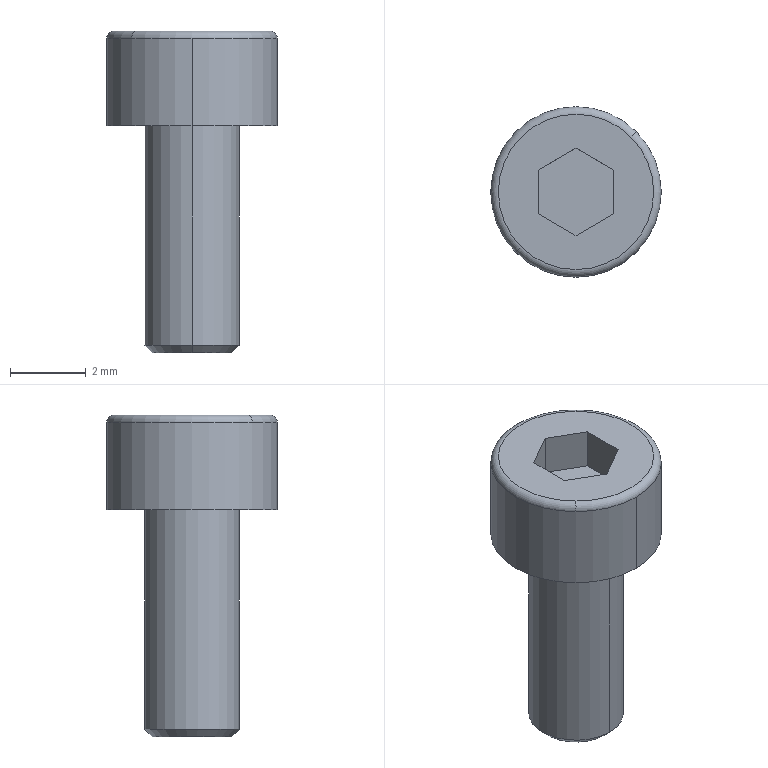Part | STEP file | ASND-0110-0211110266 | 1 solid | 18 faces | box 4.5 x 4.5 x 8.5 mm | volume 65.135 mm3 | plane 10 | cylinder 4 | torus 2 | cone 2 | commonest cylinder face diameters 2.5 x2 4.5 x2
STEP:
#1=CARTESIAN_POINT('',(0.,0.,0.));
#2=DIRECTION('',(0.,0.,1.));
#3=DIRECTION('',(1.,0.,0.));
#4=AXIS2_PLACEMENT_3D('',#1,#2,#3);
#5=CARTESIAN_POINT('',(-1.45,-1.45,2.5));
#6=VERTEX_POINT('',#5);
#7=CARTESIAN_POINT('',(1.45,1.45,2.5));
#8=VERTEX_POINT('',#7);
#9=CARTESIAN_POINT('',(0.,0.,2.5));
#10=DIRECTION('',(0.,0.,1.));
#11=DIRECTION('',(0.,-1.,0.));
#12=AXIS2_PLACEMENT_3D('',#9,#10,#11);
#13=CIRCLE('',#12,2.05);
#14=CARTESIAN_POINT('',(0.,0.,2.3));
#15=DIRECTION('',(0.,0.,-1.));
#16=DIRECTION('',(0.7071,0.7071,0.));
#17=AXIS2_PLACEMENT_3D('',#14,#15,#16);
#18=TOROIDAL_SURFACE('',#17,2.05,0.2);
#19=CARTESIAN_POINT('',(8.639,4.712));
#20=DIRECTION('',(-1.,0.));
#21=VECTOR('',#20,1.);
#22=LINE('',#19,#21);
#23=(GEOMETRIC_REPRESENTATION_CONTEXT(2)PARAMETRIC_REPRESENTATION_CONTEXT()REPRESENTATION_CONTEXT('',''));
#24=DEFINITIONAL_REPRESENTATION('',(#22),#23);
#25=PCURVE('',#18,#24);
#26=CARTESIAN_POINT('',(0.,0.,2.5));
#27=DIRECTION('',(0.,0.,-1.));
#28=DIRECTION('',(0.7071,0.7071,0.));
#29=AXIS2_PLACEMENT_3D('',#26,#27,#28);
#30=PLANE('',#29);
#31=CARTESIAN_POINT('',(-1.45,1.45));
#32=CARTESIAN_POINT('',(1.061,3.96));
#33=CARTESIAN_POINT('',(1.98,0.5306));
#34=CARTESIAN_POINT('',(2.899,-2.899));
#35=CARTESIAN_POINT('',(-0.5306,-1.98));
#36=CARTESIAN_POINT('',(-3.96,-1.061));
#37=CARTESIAN_POINT('',(-1.45,1.45));
#38=(BOUNDED_CURVE()B_SPLINE_CURVE(2,(#31,#32,#33,#34,#35,#36,#37),.UNSPECIFIED.,.T.,.F.)B_SPLINE_CURVE_WITH_KNOTS((1,2,2,2,2,1),(-2.094,0.,2.094,4.189,6.283,8.378),.UNSPECIFIED.)CURVE()GEOMETRIC_REPRESENTATION_ITEM()RATIONAL_B_SPLINE_CURVE((1.,0.5,1.,0.5,1.,0.5,1.))REPRESENTATION_ITEM(''));
#39=(GEOMETRIC_REPRESENTATION_CONTEXT(2)PARAMETRIC_REPRESENTATION_CONTEXT()REPRESENTATION_CONTEXT('',''));
#40=DEFINITIONAL_REPRESENTATION('',(#38),#39);
#41=PCURVE('',#30,#40);
#42=SURFACE_CURVE('',#13,(#25,#41),.PCURVE_S1.);
#43=EDGE_CURVE('',#6,#8,#42,.T.);
#44=ORIENTED_EDGE('',*,*,#43,.F.);
#45=CARTESIAN_POINT('',(-1.591,-1.591,2.3));
#46=VERTEX_POINT('',#45);
#47=CARTESIAN_POINT('',(-1.45,-1.45,2.3));
#48=DIRECTION('',(0.7071,-0.7071,0.));
#49=DIRECTION('',(0.7071,0.7071,0.));
#50=AXIS2_PLACEMENT_3D('',#47,#48,#49);
#51=CIRCLE('',#50,0.2);
#52=CARTESIAN_POINT('',(3.142,3.142));
#53=DIRECTION('',(0.,1.));
#54=VECTOR('',#53,1.);
#55=LINE('',#52,#54);
#56=(GEOMETRIC_REPRESENTATION_CONTEXT(2)PARAMETRIC_REPRESENTATION_CONTEXT()REPRESENTATION_CONTEXT('',''));
#57=DEFINITIONAL_REPRESENTATION('',(#55),#56);
#58=PCURVE('',#18,#57);
#59=CARTESIAN_POINT('',(0.,0.,2.3));
#60=DIRECTION('',(0.,0.,-1.));
#61=DIRECTION('',(0.7071,0.7071,0.));
#62=AXIS2_PLACEMENT_3D('',#59,#60,#61);
#63=TOROIDAL_SURFACE('',#62,2.05,0.2);
#64=CARTESIAN_POINT('',(3.142,3.142));
#65=DIRECTION('',(0.,1.));
#66=VECTOR('',#65,1.);
#67=LINE('',#64,#66);
#68=(GEOMETRIC_REPRESENTATION_CONTEXT(2)PARAMETRIC_REPRESENTATION_CONTEXT()REPRESENTATION_CONTEXT('',''));
#69=DEFINITIONAL_REPRESENTATION('',(#67),#68);
#70=PCURVE('',#63,#69);
#71=SURFACE_CURVE('',#51,(#58,#70),.PCURVE_S1.);
#72=EDGE_CURVE('',#6,#46,#71,.T.);
#73=ORIENTED_EDGE('',*,*,#72,.T.);
#74=CARTESIAN_POINT('',(0.,-2.25,2.3));
#75=VERTEX_POINT('',#74);
#76=CARTESIAN_POINT('',(0.,0.,2.3));
#77=DIRECTION('',(0.,0.,1.));
#78=DIRECTION('',(0.,-1.,0.));
#79=AXIS2_PLACEMENT_3D('',#76,#77,#78);
#80=CIRCLE('',#79,2.25);
#81=CARTESIAN_POINT('',(8.639,6.283));
#82=DIRECTION('',(-1.,0.));
#83=VECTOR('',#82,1.);
#84=LINE('',#81,#83);
#85=(GEOMETRIC_REPRESENTATION_CONTEXT(2)PARAMETRIC_REPRESENTATION_CONTEXT()REPRESENTATION_CONTEXT('',''));
#86=DEFINITIONAL_REPRESENTATION('',(#84),#85);
#87=PCURVE('',#18,#86);
#88=CARTESIAN_POINT('',(0.,0.,2.925));
#89=DIRECTION('',(0.,0.,-1.));
#90=DIRECTION('',(0.,1.,0.));
#91=AXIS2_PLACEMENT_3D('',#88,#89,#90);
#92=CYLINDRICAL_SURFACE('',#91,2.25);
#93=CARTESIAN_POINT('',(9.425,0.625));
#94=DIRECTION('',(-1.,0.));
#95=VECTOR('',#94,1.);
#96=LINE('',#93,#95);
#97=(GEOMETRIC_REPRESENTATION_CONTEXT(2)PARAMETRIC_REPRESENTATION_CONTEXT()REPRESENTATION_CONTEXT('',''));
#98=DEFINITIONAL_REPRESENTATION('',(#96),#97);
#99=PCURVE('',#92,#98);
#100=SURFACE_CURVE('',#80,(#87,#99),.PCURVE_S1.);
#101=EDGE_CURVE('',#46,#75,#100,.T.);
#102=ORIENTED_EDGE('',*,*,#101,.T.);
#103=CARTESIAN_POINT('',(1.591,1.591,2.3));
#104=VERTEX_POINT('',#103);
#105=CARTESIAN_POINT('',(0.,0.,2.3));
#106=DIRECTION('',(0.,0.,1.));
#107=DIRECTION('',(0.,-1.,0.));
#108=AXIS2_PLACEMENT_3D('',#105,#106,#107);
#109=CIRCLE('',#108,2.25);
#110=CARTESIAN_POINT('',(2.356,6.283));
#111=DIRECTION('',(-1.,0.));
#112=VECTOR('',#111,1.);
#113=LINE('',#110,#112);
#114=(GEOMETRIC_REPRESENTATION_CONTEXT(2)PARAMETRIC_REPRESENTATION_CONTEXT()REPRESENTATION_CONTEXT('',''));
#115=DEFINITIONAL_REPRESENTATION('',(#113),#114);
#116=PCURVE('',#18,#115);
#117=CARTESIAN_POINT('',(0.,0.,2.925));
#118=DIRECTION('',(0.,0.,-1.));
#119=DIRECTION('',(0.,1.,0.));
#120=AXIS2_PLACEMENT_3D('',#117,#118,#119);
#121=CYLINDRICAL_SURFACE('',#120,2.25);
#122=CARTESIAN_POINT('',(3.142,0.625));
#123=DIRECTION('',(-1.,0.));
#124=VECTOR('',#123,1.);
#125=LINE('',#122,#124);
#126=(GEOMETRIC_REPRESENTATION_CONTEXT(2)PARAMETRIC_REPRESENTATION_CONTEXT()REPRESENTATION_CONTEXT('',''));
#127=DEFINITIONAL_REPRESENTATION('',(#125),#126);
#128=PCURVE('',#121,#127);
#129=SURFACE_CURVE('',#109,(#116,#128),.PCURVE_S1.);
#130=EDGE_CURVE('',#75,#104,#129,.T.);
#131=ORIENTED_EDGE('',*,*,#130,.T.);
#132=CARTESIAN_POINT('',(1.45,1.45,2.3));
#133=DIRECTION('',(-0.7071,0.7071,0.));
#134=DIRECTION('',(-0.7071,-0.7071,0.));
#135=AXIS2_PLACEMENT_3D('',#132,#133,#134);
#136=CIRCLE('',#135,0.2);
#137=CARTESIAN_POINT('',(0.,3.142));
#138=DIRECTION('',(0.,1.));
#139=VECTOR('',#138,1.);
#140=LINE('',#137,#139);
#141=(GEOMETRIC_REPRESENTATION_CONTEXT(2)PARAMETRIC_REPRESENTATION_CONTEXT()REPRESENTATION_CONTEXT('',''));
#142=DEFINITIONAL_REPRESENTATION('',(#140),#141);
#143=PCURVE('',#18,#142);
#144=CARTESIAN_POINT('',(6.283,3.142));
#145=DIRECTION('',(0.,1.));
#146=VECTOR('',#145,1.);
#147=LINE('',#144,#146);
#148=(GEOMETRIC_REPRESENTATION_CONTEXT(2)PARAMETRIC_REPRESENTATION_CONTEXT()REPRESENTATION_CONTEXT('',''));
#149=DEFINITIONAL_REPRESENTATION('',(#147),#148);
#150=PCURVE('',#63,#149);
#151=SURFACE_CURVE('',#136,(#143,#150),.PCURVE_S1.);
#152=EDGE_CURVE('',#8,#104,#151,.T.);
#153=ORIENTED_EDGE('',*,*,#152,.F.);
#154=EDGE_LOOP('',(#44,#73,#102,#131,#153));
#155=FACE_BOUND('',#154,.T.);
#156=ADVANCED_FACE('',(#155),#18,.T.);
#157=ORIENTED_EDGE('',*,*,#130,.F.);
#158=CARTESIAN_POINT('',(0.,-2.25,0.));
#159=VERTEX_POINT('',#158);
#160=CARTESIAN_POINT('',(0.,-2.25,2.925));
#161=DIRECTION('',(0.,0.,-1.));
#162=VECTOR('',#161,1.);
#163=LINE('',#160,#162);
#164=CARTESIAN_POINT('',(3.142,0.));
#165=DIRECTION('',(0.,1.));
#166=VECTOR('',#165,1.);
#167=LINE('',#164,#166);
#168=(GEOMETRIC_REPRESENTATION_CONTEXT(2)PARAMETRIC_REPRESENTATION_CONTEXT()REPRESENTATION_CONTEXT('',''));
#169=DEFINITIONAL_REPRESENTATION('',(#167),#168);
#170=PCURVE('',#121,#169);
#171=CARTESIAN_POINT('',(3.142,0.));
#172=DIRECTION('',(0.,1.));
#173=VECTOR('',#172,1.);
#174=LINE('',#171,#173);
#175=(GEOMETRIC_REPRESENTATION_CONTEXT(2)PARAMETRIC_REPRESENTATION_CONTEXT()REPRESENTATION_CONTEXT('',''));
#176=DEFINITIONAL_REPRESENTATION('',(#174),#175);
#177=PCURVE('',#92,#176);
#178=SURFACE_CURVE('',#163,(#170,#177),.PCURVE_S1.);
#179=EDGE_CURVE('',#75,#159,#178,.T.);
#180=ORIENTED_EDGE('',*,*,#179,.T.);
#181=CARTESIAN_POINT('',(0.,2.25,0.));
#182=VERTEX_POINT('',#181);
#183=CARTESIAN_POINT('',(0.,0.,0.));
#184=DIRECTION('',(0.,0.,1.));
#185=DIRECTION('',(0.,-1.,0.));
#186=AXIS2_PLACEMENT_3D('',#183,#184,#185);
#187=CIRCLE('',#186,2.25);
#188=CARTESIAN_POINT('',(3.142,2.925));
#189=DIRECTION('',(-1.,0.));
#190=VECTOR('',#189,1.);
#191=LINE('',#188,#190);
#192=(GEOMETRIC_REPRESENTATION_CONTEXT(2)PARAMETRIC_REPRESENTATION_CONTEXT()REPRESENTATION_CONTEXT('',''));
#193=DEFINITIONAL_REPRESENTATION('',(#191),#192);
#194=PCURVE('',#121,#193);
#195=CARTESIAN_POINT('',(0.,0.,0.));
#196=DIRECTION('',(0.,0.,-1.));
#197=DIRECTION('',(0.7071,0.7071,0.));
#198=AXIS2_PLACEMENT_3D('',#195,#196,#197);
#199=PLANE('',#198);
#200=CARTESIAN_POINT('',(-1.591,1.591));
#201=CARTESIAN_POINT('',(1.165,4.347));
#202=CARTESIAN_POINT('',(2.173,0.5823));
#203=CARTESIAN_POINT('',(3.182,-3.182));
#204=CARTESIAN_POINT('',(-0.5823,-2.173));
#205=CARTESIAN_POINT('',(-4.347,-1.165));
#206=CARTESIAN_POINT('',(-1.591,1.591));
#207=(BOUNDED_CURVE()B_SPLINE_CURVE(2,(#200,#201,#202,#203,#204,#205,#206),.UNSPECIFIED.,.T.,.F.)B_SPLINE_CURVE_WITH_KNOTS((1,2,2,2,2,1),(-2.094,0.,2.094,4.189,6.283,8.378),.UNSPECIFIED.)CURVE()GEOMETRIC_REPRESENTATION_ITEM()RATIONAL_B_SPLINE_CURVE((1.,0.5,1.,0.5,1.,0.5,1.))REPRESENTATION_ITEM(''));
#208=(GEOMETRIC_REPRESENTATION_CONTEXT(2)PARAMETRIC_REPRESENTATION_CONTEXT()REPRESENTATION_CONTEXT('',''));
#209=DEFINITIONAL_REPRESENTATION('',(#207),#208);
#210=PCURVE('',#199,#209);
#211=SURFACE_CURVE('',#187,(#194,#210),.PCURVE_S1.);
#212=EDGE_CURVE('',#159,#182,#211,.T.);
#213=ORIENTED_EDGE('',*,*,#212,.T.);
#214=CARTESIAN_POINT('',(0.,2.25,2.3));
#215=VERTEX_POINT('',#214);
#216=CARTESIAN_POINT('',(0.,2.25,2.925));
#217=DIRECTION('',(0.,0.,-1.));
#218=VECTOR('',#217,1.);
#219=LINE('',#216,#218);
#220=CARTESIAN_POINT('',(0.,0.));
#221=DIRECTION('',(0.,1.));
#222=VECTOR('',#221,1.);
#223=LINE('',#220,#222);
#224=(GEOMETRIC_REPRESENTATION_CONTEXT(2)PARAMETRIC_REPRESENTATION_CONTEXT()REPRESENTATION_CONTEXT('',''));
#225=DEFINITIONAL_REPRESENTATION('',(#223),#224);
#226=PCURVE('',#121,#225);
#227=CARTESIAN_POINT('',(6.283,0.));
#228=DIRECTION('',(0.,1.));
#229=VECTOR('',#228,1.);
#230=LINE('',#227,#229);
#231=(GEOMETRIC_REPRESENTATION_CONTEXT(2)PARAMETRIC_REPRESENTATION_CONTEXT()REPRESENTATION_CONTEXT('',''));
#232=DEFINITIONAL_REPRESENTATION('',(#230),#231);
#233=PCURVE('',#92,#232);
#234=SURFACE_CURVE('',#219,(#226,#233),.PCURVE_S1.);
#235=EDGE_CURVE('',#215,#182,#234,.T.);
#236=ORIENTED_EDGE('',*,*,#235,.F.);
#237=CARTESIAN_POINT('',(0.,0.,2.3));
#238=DIRECTION('',(0.,0.,1.));
#239=DIRECTION('',(0.,-1.,0.));
#240=AXIS2_PLACEMENT_3D('',#237,#238,#239);
#241=CIRCLE('',#240,2.25);
#242=CARTESIAN_POINT('',(3.142,0.625));
#243=DIRECTION('',(-1.,0.));
#244=VECTOR('',#243,1.);
#245=LINE('',#242,#244);
#246=(GEOMETRIC_REPRESENTATION_CONTEXT(2)PARAMETRIC_REPRESENTATION_CONTEXT()REPRESENTATION_CONTEXT('',''));
#247=DEFINITIONAL_REPRESENTATION('',(#245),#246);
#248=PCURVE('',#121,#247);
#249=CARTESIAN_POINT('',(8.639,6.283));
#250=DIRECTION('',(-1.,0.));
#251=VECTOR('',#250,1.);
#252=LINE('',#249,#251);
#253=(GEOMETRIC_REPRESENTATION_CONTEXT(2)PARAMETRIC_REPRESENTATION_CONTEXT()REPRESENTATION_CONTEXT('',''));
#254=DEFINITIONAL_REPRESENTATION('',(#252),#253);
#255=PCURVE('',#63,#254);
#256=SURFACE_CURVE('',#241,(#248,#255),.PCURVE_S1.);
#257=EDGE_CURVE('',#104,#215,#256,.T.);
#258=ORIENTED_EDGE('',*,*,#257,.F.);
#259=EDGE_LOOP('',(#157,#180,#213,#236,#258));
#260=FACE_BOUND('',#259,.T.);
#261=ADVANCED_FACE('',(#260),#121,.T.);
#262=CARTESIAN_POINT('',(0.,1.25,0.));
#263=VERTEX_POINT('',#262);
#264=CARTESIAN_POINT('',(0.,-1.25,0.));
#265=VERTEX_POINT('',#264);
#266=CARTESIAN_POINT('',(0.,0.,0.));
#267=DIRECTION('',(0.,0.,-1.));
#268=DIRECTION('',(0.,-1.,0.));
#269=AXIS2_PLACEMENT_3D('',#266,#267,#268);
#270=CIRCLE('',#269,1.25);
#271=CARTESIAN_POINT('',(0.,0.,2.925));
#272=DIRECTION('',(0.,0.,-1.));
#273=DIRECTION('',(0.,1.,0.));
#274=AXIS2_PLACEMENT_3D('',#271,#272,#273);
#275=CYLINDRICAL_SURFACE('',#274,1.25);
#276=CARTESIAN_POINT('',(-3.142,2.925));
#277=DIRECTION('',(1.,0.));
#278=VECTOR('',#277,1.);
#279=LINE('',#276,#278);
#280=(GEOMETRIC_REPRESENTATION_CONTEXT(2)PARAMETRIC_REPRESENTATION_CONTEXT()REPRESENTATION_CONTEXT('',''));
#281=DEFINITIONAL_REPRESENTATION('',(#279),#280);
#282=PCURVE('',#275,#281);
#283=CARTESIAN_POINT('',(0.,0.));
#284=DIRECTION('',(-0.7071,0.7071));
#285=AXIS2_PLACEMENT_2D('',#283,#284);
#286=CIRCLE('',#285,1.25);
#287=(GEOMETRIC_REPRESENTATION_CONTEXT(2)PARAMETRIC_REPRESENTATION_CONTEXT()REPRESENTATION_CONTEXT('',''));
#288=DEFINITIONAL_REPRESENTATION('',(#286),#287);
#289=PCURVE('',#199,#288);
#290=SURFACE_CURVE('',#270,(#282,#289),.PCURVE_S1.);
#291=EDGE_CURVE('',#263,#265,#290,.T.);
#292=ORIENTED_EDGE('',*,*,#291,.T.);
#293=CARTESIAN_POINT('',(0.,-1.25,-5.8));
#294=VERTEX_POINT('',#293);
#295=CARTESIAN_POINT('',(0.,-1.25,2.925));
#296=DIRECTION('',(0.,0.,-1.));
#297=VECTOR('',#296,1.);
#298=LINE('',#295,#297);
#299=CARTESIAN_POINT('',(3.142,0.));
#300=DIRECTION('',(0.,1.));
#301=VECTOR('',#300,1.);
#302=LINE('',#299,#301);
#303=(GEOMETRIC_REPRESENTATION_CONTEXT(2)PARAMETRIC_REPRESENTATION_CONTEXT()REPRESENTATION_CONTEXT('',''));
#304=DEFINITIONAL_REPRESENTATION('',(#302),#303);
#305=PCURVE('',#275,#304);
#306=CARTESIAN_POINT('',(0.,0.,2.925));
#307=DIRECTION('',(0.,0.,-1.));
#308=DIRECTION('',(0.,1.,0.));
#309=AXIS2_PLACEMENT_3D('',#306,#307,#308);
#310=CYLINDRICAL_SURFACE('',#309,1.25);
#311=CARTESIAN_POINT('',(3.142,0.));
#312=DIRECTION('',(0.,1.));
#313=VECTOR('',#312,1.);
#314=LINE('',#311,#313);
#315=(GEOMETRIC_REPRESENTATION_CONTEXT(2)PARAMETRIC_REPRESENTATION_CONTEXT()REPRESENTATION_CONTEXT('',''));
#316=DEFINITIONAL_REPRESENTATION('',(#314),#315);
#317=PCURVE('',#310,#316);
#318=SURFACE_CURVE('',#298,(#305,#317),.PCURVE_S1.);
#319=EDGE_CURVE('',#265,#294,#318,.T.);
#320=ORIENTED_EDGE('',*,*,#319,.T.);
#321=CARTESIAN_POINT('',(0.,1.25,-5.8));
#322=VERTEX_POINT('',#321);
#323=CARTESIAN_POINT('',(0.,0.,-5.8));
#324=DIRECTION('',(0.,0.,1.));
#325=DIRECTION('',(0.,1.,0.));
#326=AXIS2_PLACEMENT_3D('',#323,#324,#325);
#327=CIRCLE('',#326,1.25);
#328=CARTESIAN_POINT('',(6.283,8.725));
#329=DIRECTION('',(-1.,0.));
#330=VECTOR('',#329,1.);
#331=LINE('',#328,#330);
#332=(GEOMETRIC_REPRESENTATION_CONTEXT(2)PARAMETRIC_REPRESENTATION_CONTEXT()REPRESENTATION_CONTEXT('',''));
#333=DEFINITIONAL_REPRESENTATION('',(#331),#332);
#334=PCURVE('',#275,#333);
#335=CARTESIAN_POINT('',(0.,0.,-5.9));
#336=DIRECTION('',(0.,0.,1.));
#337=DIRECTION('',(0.,-1.,0.));
#338=AXIS2_PLACEMENT_3D('',#335,#336,#337);
#339=CONICAL_SURFACE('',#338,1.15,0.7854);
#340=CARTESIAN_POINT('',(-3.142,0.1));
#341=DIRECTION('',(1.,0.));
#342=VECTOR('',#341,1.);
#343=LINE('',#340,#342);
#344=(GEOMETRIC_REPRESENTATION_CONTEXT(2)PARAMETRIC_REPRESENTATION_CONTEXT()REPRESENTATION_CONTEXT('',''));
#345=DEFINITIONAL_REPRESENTATION('',(#343),#344);
#346=PCURVE('',#339,#345);
#347=SURFACE_CURVE('',#327,(#334,#346),.PCURVE_S1.);
#348=EDGE_CURVE('',#294,#322,#347,.T.);
#349=ORIENTED_EDGE('',*,*,#348,.T.);
#350=CARTESIAN_POINT('',(0.,1.25,2.925));
#351=DIRECTION('',(0.,0.,-1.));
#352=VECTOR('',#351,1.);
#353=LINE('',#350,#352);
#354=CARTESIAN_POINT('',(0.,0.));
#355=DIRECTION('',(0.,1.));
#356=VECTOR('',#355,1.);
#357=LINE('',#354,#356);
#358=(GEOMETRIC_REPRESENTATION_CONTEXT(2)PARAMETRIC_REPRESENTATION_CONTEXT()REPRESENTATION_CONTEXT('',''));
#359=DEFINITIONAL_REPRESENTATION('',(#357),#358);
#360=PCURVE('',#275,#359);
#361=CARTESIAN_POINT('',(6.283,0.));
#362=DIRECTION('',(0.,1.));
#363=VECTOR('',#362,1.);
#364=LINE('',#361,#363);
#365=(GEOMETRIC_REPRESENTATION_CONTEXT(2)PARAMETRIC_REPRESENTATION_CONTEXT()REPRESENTATION_CONTEXT('',''));
#366=DEFINITIONAL_REPRESENTATION('',(#364),#365);
#367=PCURVE('',#310,#366);
#368=SURFACE_CURVE('',#353,(#360,#367),.PCURVE_S1.);
#369=EDGE_CURVE('',#263,#322,#368,.T.);
#370=ORIENTED_EDGE('',*,*,#369,.F.);
#371=EDGE_LOOP('',(#292,#320,#349,#370));
#372=FACE_BOUND('',#371,.T.);
#373=ADVANCED_FACE('',(#372),#275,.T.);
#374=CARTESIAN_POINT('',(0.,-1.05,-6.));
#375=VERTEX_POINT('',#374);
#376=CARTESIAN_POINT('',(0.,1.05,-6.));
#377=VERTEX_POINT('',#376);
#378=CARTESIAN_POINT('',(0.,0.,-6.));
#379=DIRECTION('',(0.,0.,1.));
#380=DIRECTION('',(0.,1.,0.));
#381=AXIS2_PLACEMENT_3D('',#378,#379,#380);
#382=CIRCLE('',#381,1.05);
#383=CARTESIAN_POINT('',(-3.142,-0.1));
#384=DIRECTION('',(1.,0.));
#385=VECTOR('',#384,1.);
#386=LINE('',#383,#385);
#387=(GEOMETRIC_REPRESENTATION_CONTEXT(2)PARAMETRIC_REPRESENTATION_CONTEXT()REPRESENTATION_CONTEXT('',''));
#388=DEFINITIONAL_REPRESENTATION('',(#386),#387);
#389=PCURVE('',#339,#388);
#390=CARTESIAN_POINT('',(0.,0.,-6.));
#391=DIRECTION('',(0.,0.,-1.));
#392=DIRECTION('',(0.7071,0.7071,0.));
#393=AXIS2_PLACEMENT_3D('',#390,#391,#392);
#394=PLANE('',#393);
#395=CARTESIAN_POINT('',(0.7425,-0.7425));
#396=CARTESIAN_POINT('',(-0.5435,-2.028));
#397=CARTESIAN_POINT('',(-1.014,-0.2718));
#398=CARTESIAN_POINT('',(-1.485,1.485));
#399=CARTESIAN_POINT('',(0.2718,1.014));
#400=CARTESIAN_POINT('',(2.028,0.5435));
#401=CARTESIAN_POINT('',(0.7425,-0.7425));
#402=(BOUNDED_CURVE()B_SPLINE_CURVE(2,(#395,#396,#397,#398,#399,#400,#401),.UNSPECIFIED.,.T.,.F.)B_SPLINE_CURVE_WITH_KNOTS((1,2,2,2,2,1),(-2.094,0.,2.094,4.189,6.283,8.378),.UNSPECIFIED.)CURVE()GEOMETRIC_REPRESENTATION_ITEM()RATIONAL_B_SPLINE_CURVE((1.,0.5,1.,0.5,1.,0.5,1.))REPRESENTATION_ITEM(''));
#403=(GEOMETRIC_REPRESENTATION_CONTEXT(2)PARAMETRIC_REPRESENTATION_CONTEXT()REPRESENTATION_CONTEXT('',''));
#404=DEFINITIONAL_REPRESENTATION('',(#402),#403);
#405=PCURVE('',#394,#404);
#406=SURFACE_CURVE('',#382,(#389,#405),.PCURVE_S1.);
#407=EDGE_CURVE('',#375,#377,#406,.T.);
#408=ORIENTED_EDGE('',*,*,#407,.T.);
#409=CARTESIAN_POINT('',(0.,1.15,-5.9));
#410=DIRECTION('',(0.,0.7071,0.7071));
#411=VECTOR('',#410,1.);
#412=LINE('',#409,#411);
#413=CARTESIAN_POINT('',(3.142,0.));
#414=DIRECTION('',(0.,1.));
#415=VECTOR('',#414,1.);
#416=LINE('',#413,#415);
#417=(GEOMETRIC_REPRESENTATION_CONTEXT(2)PARAMETRIC_REPRESENTATION_CONTEXT()REPRESENTATION_CONTEXT('',''));
#418=DEFINITIONAL_REPRESENTATION('',(#416),#417);
#419=PCURVE('',#339,#418);
#420=CARTESIAN_POINT('',(0.,0.,-5.9));
#421=DIRECTION('',(0.,0.,1.));
#422=DIRECTION('',(0.,-1.,0.));
#423=AXIS2_PLACEMENT_3D('',#420,#421,#422);
#424=CONICAL_SURFACE('',#423,1.15,0.7854);
#425=CARTESIAN_POINT('',(3.142,0.));
#426=DIRECTION('',(0.,1.));
#427=VECTOR('',#426,1.);
#428=LINE('',#425,#427);
#429=(GEOMETRIC_REPRESENTATION_CONTEXT(2)PARAMETRIC_REPRESENTATION_CONTEXT()REPRESENTATION_CONTEXT('',''));
#430=DEFINITIONAL_REPRESENTATION('',(#428),#429);
#431=PCURVE('',#424,#430);
#432=SURFACE_CURVE('',#412,(#419,#431),.PCURVE_S1.);
#433=EDGE_CURVE('',#377,#322,#432,.T.);
#434=ORIENTED_EDGE('',*,*,#433,.T.);
#435=ORIENTED_EDGE('',*,*,#348,.F.);
#436=CARTESIAN_POINT('',(0.,-1.15,-5.9));
#437=DIRECTION('',(0.,-0.7071,0.7071));
#438=VECTOR('',#437,1.);
#439=LINE('',#436,#438);
#440=CARTESIAN_POINT('',(0.,0.));
#441=DIRECTION('',(0.,1.));
#442=VECTOR('',#441,1.);
#443=LINE('',#440,#442);
#444=(GEOMETRIC_REPRESENTATION_CONTEXT(2)PARAMETRIC_REPRESENTATION_CONTEXT()REPRESENTATION_CONTEXT('',''));
#445=DEFINITIONAL_REPRESENTATION('',(#443),#444);
#446=PCURVE('',#339,#445);
#447=CARTESIAN_POINT('',(6.283,0.));
#448=DIRECTION('',(0.,1.));
#449=VECTOR('',#448,1.);
#450=LINE('',#447,#449);
#451=(GEOMETRIC_REPRESENTATION_CONTEXT(2)PARAMETRIC_REPRESENTATION_CONTEXT()REPRESENTATION_CONTEXT('',''));
#452=DEFINITIONAL_REPRESENTATION('',(#450),#451);
#453=PCURVE('',#424,#452);
#454=SURFACE_CURVE('',#439,(#446,#453),.PCURVE_S1.);
#455=EDGE_CURVE('',#375,#294,#454,.T.);
#456=ORIENTED_EDGE('',*,*,#455,.F.);
#457=EDGE_LOOP('',(#408,#434,#435,#456));
#458=FACE_BOUND('',#457,.T.);
#459=ADVANCED_FACE('',(#458),#339,.T.);
#460=ORIENTED_EDGE('',*,*,#407,.F.);
#461=CARTESIAN_POINT('',(0.,0.,-6.));
#462=DIRECTION('',(0.,0.,1.));
#463=DIRECTION('',(0.,1.,0.));
#464=AXIS2_PLACEMENT_3D('',#461,#462,#463);
#465=CIRCLE('',#464,1.05);
#466=CARTESIAN_POINT('',(0.7425,-0.7425));
#467=CARTESIAN_POINT('',(-0.5435,-2.028));
#468=CARTESIAN_POINT('',(-1.014,-0.2718));
#469=CARTESIAN_POINT('',(-1.485,1.485));
#470=CARTESIAN_POINT('',(0.2718,1.014));
#471=CARTESIAN_POINT('',(2.028,0.5435));
#472=CARTESIAN_POINT('',(0.7425,-0.7425));
#473=(BOUNDED_CURVE()B_SPLINE_CURVE(2,(#466,#467,#468,#469,#470,#471,#472),.UNSPECIFIED.,.T.,.F.)B_SPLINE_CURVE_WITH_KNOTS((1,2,2,2,2,1),(-2.094,0.,2.094,4.189,6.283,8.378),.UNSPECIFIED.)CURVE()GEOMETRIC_REPRESENTATION_ITEM()RATIONAL_B_SPLINE_CURVE((1.,0.5,1.,0.5,1.,0.5,1.))REPRESENTATION_ITEM(''));
#474=(GEOMETRIC_REPRESENTATION_CONTEXT(2)PARAMETRIC_REPRESENTATION_CONTEXT()REPRESENTATION_CONTEXT('',''));
#475=DEFINITIONAL_REPRESENTATION('',(#473),#474);
#476=PCURVE('',#394,#475);
#477=CARTESIAN_POINT('',(3.142,-0.1));
#478=DIRECTION('',(1.,0.));
#479=VECTOR('',#478,1.);
#480=LINE('',#477,#479);
#481=(GEOMETRIC_REPRESENTATION_CONTEXT(2)PARAMETRIC_REPRESENTATION_CONTEXT()REPRESENTATION_CONTEXT('',''));
#482=DEFINITIONAL_REPRESENTATION('',(#480),#481);
#483=PCURVE('',#424,#482);
#484=SURFACE_CURVE('',#465,(#476,#483),.PCURVE_S1.);
#485=EDGE_CURVE('',#377,#375,#484,.T.);
#486=ORIENTED_EDGE('',*,*,#485,.F.);
#487=EDGE_LOOP('',(#460,#486));
#488=FACE_BOUND('',#487,.T.);
#489=ADVANCED_FACE('',(#488),#394,.T.);
#490=ORIENTED_EDGE('',*,*,#433,.F.);
#491=ORIENTED_EDGE('',*,*,#485,.T.);
#492=ORIENTED_EDGE('',*,*,#455,.T.);
#493=CARTESIAN_POINT('',(0.,0.,-5.8));
#494=DIRECTION('',(0.,0.,1.));
#495=DIRECTION('',(0.,1.,0.));
#496=AXIS2_PLACEMENT_3D('',#493,#494,#495);
#497=CIRCLE('',#496,1.25);
#498=CARTESIAN_POINT('',(3.142,0.1));
#499=DIRECTION('',(1.,0.));
#500=VECTOR('',#499,1.);
#501=LINE('',#498,#500);
#502=(GEOMETRIC_REPRESENTATION_CONTEXT(2)PARAMETRIC_REPRESENTATION_CONTEXT()REPRESENTATION_CONTEXT('',''));
#503=DEFINITIONAL_REPRESENTATION('',(#501),#502);
#504=PCURVE('',#424,#503);
#505=CARTESIAN_POINT('',(6.283,8.725));
#506=DIRECTION('',(-1.,0.));
#507=VECTOR('',#506,1.);
#508=LINE('',#505,#507);
#509=(GEOMETRIC_REPRESENTATION_CONTEXT(2)PARAMETRIC_REPRESENTATION_CONTEXT()REPRESENTATION_CONTEXT('',''));
#510=DEFINITIONAL_REPRESENTATION('',(#508),#509);
#511=PCURVE('',#310,#510);
#512=SURFACE_CURVE('',#497,(#504,#511),.PCURVE_S1.);
#513=EDGE_CURVE('',#322,#294,#512,.T.);
#514=ORIENTED_EDGE('',*,*,#513,.F.);
#515=EDGE_LOOP('',(#490,#491,#492,#514));
#516=FACE_BOUND('',#515,.T.);
#517=ADVANCED_FACE('',(#516),#424,.T.);
#518=ORIENTED_EDGE('',*,*,#319,.F.);
#519=CARTESIAN_POINT('',(0.,0.,0.));
#520=DIRECTION('',(0.,0.,-1.));
#521=DIRECTION('',(0.,-1.,0.));
#522=AXIS2_PLACEMENT_3D('',#519,#520,#521);
#523=CIRCLE('',#522,1.25);
#524=CARTESIAN_POINT('',(3.142,2.925));
#525=DIRECTION('',(1.,0.));
#526=VECTOR('',#525,1.);
#527=LINE('',#524,#526);
#528=(GEOMETRIC_REPRESENTATION_CONTEXT(2)PARAMETRIC_REPRESENTATION_CONTEXT()REPRESENTATION_CONTEXT('',''));
#529=DEFINITIONAL_REPRESENTATION('',(#527),#528);
#530=PCURVE('',#310,#529);
#531=CARTESIAN_POINT('',(0.,0.));
#532=DIRECTION('',(-0.7071,0.7071));
#533=AXIS2_PLACEMENT_2D('',#531,#532);
#534=CIRCLE('',#533,1.25);
#535=(GEOMETRIC_REPRESENTATION_CONTEXT(2)PARAMETRIC_REPRESENTATION_CONTEXT()REPRESENTATION_CONTEXT('',''));
#536=DEFINITIONAL_REPRESENTATION('',(#534),#535);
#537=PCURVE('',#199,#536);
#538=SURFACE_CURVE('',#523,(#530,#537),.PCURVE_S1.);
#539=EDGE_CURVE('',#265,#263,#538,.T.);
#540=ORIENTED_EDGE('',*,*,#539,.T.);
#541=ORIENTED_EDGE('',*,*,#369,.T.);
#542=ORIENTED_EDGE('',*,*,#513,.T.);
#543=EDGE_LOOP('',(#518,#540,#541,#542));
#544=FACE_BOUND('',#543,.T.);
#545=ADVANCED_FACE('',(#544),#310,.T.);
#546=CARTESIAN_POINT('',(0.,0.,0.));
#547=DIRECTION('',(0.,0.,1.));
#548=DIRECTION('',(0.,-1.,0.));
#549=AXIS2_PLACEMENT_3D('',#546,#547,#548);
#550=CIRCLE('',#549,2.25);
#551=CARTESIAN_POINT('',(-1.591,1.591));
#552=CARTESIAN_POINT('',(1.165,4.347));
#553=CARTESIAN_POINT('',(2.173,0.5823));
#554=CARTESIAN_POINT('',(3.182,-3.182));
#555=CARTESIAN_POINT('',(-0.5823,-2.173));
#556=CARTESIAN_POINT('',(-4.347,-1.165));
#557=CARTESIAN_POINT('',(-1.591,1.591));
#558=(BOUNDED_CURVE()B_SPLINE_CURVE(2,(#551,#552,#553,#554,#555,#556,#557),.UNSPECIFIED.,.T.,.F.)B_SPLINE_CURVE_WITH_KNOTS((1,2,2,2,2,1),(-2.094,0.,2.094,4.189,6.283,8.378),.UNSPECIFIED.)CURVE()GEOMETRIC_REPRESENTATION_ITEM()RATIONAL_B_SPLINE_CURVE((1.,0.5,1.,0.5,1.,0.5,1.))REPRESENTATION_ITEM(''));
#559=(GEOMETRIC_REPRESENTATION_CONTEXT(2)PARAMETRIC_REPRESENTATION_CONTEXT()REPRESENTATION_CONTEXT('',''));
#560=DEFINITIONAL_REPRESENTATION('',(#558),#559);
#561=PCURVE('',#199,#560);
#562=CARTESIAN_POINT('',(9.425,2.925));
#563=DIRECTION('',(-1.,0.));
#564=VECTOR('',#563,1.);
#565=LINE('',#562,#564);
#566=(GEOMETRIC_REPRESENTATION_CONTEXT(2)PARAMETRIC_REPRESENTATION_CONTEXT()REPRESENTATION_CONTEXT('',''));
#567=DEFINITIONAL_REPRESENTATION('',(#565),#566);
#568=PCURVE('',#92,#567);
#569=SURFACE_CURVE('',#550,(#561,#568),.PCURVE_S1.);
#570=EDGE_CURVE('',#182,#159,#569,.T.);
#571=ORIENTED_EDGE('',*,*,#570,.F.);
#572=ORIENTED_EDGE('',*,*,#212,.F.);
#573=EDGE_LOOP('',(#571,#572));
#574=FACE_BOUND('',#573,.T.);
#575=ORIENTED_EDGE('',*,*,#291,.F.);
#576=ORIENTED_EDGE('',*,*,#539,.F.);
#577=EDGE_LOOP('',(#575,#576));
#578=FACE_BOUND('',#577,.T.);
#579=ADVANCED_FACE('',(#574,#578),#199,.T.);
#580=ORIENTED_EDGE('',*,*,#179,.F.);
#581=ORIENTED_EDGE('',*,*,#101,.F.);
#582=CARTESIAN_POINT('',(0.,0.,2.3));
#583=DIRECTION('',(0.,0.,1.));
#584=DIRECTION('',(0.,-1.,0.));
#585=AXIS2_PLACEMENT_3D('',#582,#583,#584);
#586=CIRCLE('',#585,2.25);
#587=CARTESIAN_POINT('',(9.425,0.625));
#588=DIRECTION('',(-1.,0.));
#589=VECTOR('',#588,1.);
#590=LINE('',#587,#589);
#591=(GEOMETRIC_REPRESENTATION_CONTEXT(2)PARAMETRIC_REPRESENTATION_CONTEXT()REPRESENTATION_CONTEXT('',''));
#592=DEFINITIONAL_REPRESENTATION('',(#590),#591);
#593=PCURVE('',#92,#592);
#594=CARTESIAN_POINT('',(8.639,6.283));
#595=DIRECTION('',(-1.,0.));
#596=VECTOR('',#595,1.);
#597=LINE('',#594,#596);
#598=(GEOMETRIC_REPRESENTATION_CONTEXT(2)PARAMETRIC_REPRESENTATION_CONTEXT()REPRESENTATION_CONTEXT('',''));
#599=DEFINITIONAL_REPRESENTATION('',(#597),#598);
#600=PCURVE('',#63,#599);
#601=SURFACE_CURVE('',#586,(#593,#600),.PCURVE_S1.);
#602=EDGE_CURVE('',#215,#46,#601,.T.);
#603=ORIENTED_EDGE('',*,*,#602,.F.);
#604=ORIENTED_EDGE('',*,*,#235,.T.);
#605=ORIENTED_EDGE('',*,*,#570,.T.);
#606=EDGE_LOOP('',(#580,#581,#603,#604,#605));
#607=FACE_BOUND('',#606,.T.);
#608=ADVANCED_FACE('',(#607),#92,.T.);
#609=ORIENTED_EDGE('',*,*,#72,.F.);
#610=CARTESIAN_POINT('',(0.,0.,2.5));
#611=DIRECTION('',(0.,0.,1.));
#612=DIRECTION('',(0.,-1.,0.));
#613=AXIS2_PLACEMENT_3D('',#610,#611,#612);
#614=CIRCLE('',#613,2.05);
#615=CARTESIAN_POINT('',(8.639,4.712));
#616=DIRECTION('',(-1.,0.));
#617=VECTOR('',#616,1.);
#618=LINE('',#615,#617);
#619=(GEOMETRIC_REPRESENTATION_CONTEXT(2)PARAMETRIC_REPRESENTATION_CONTEXT()REPRESENTATION_CONTEXT('',''));
#620=DEFINITIONAL_REPRESENTATION('',(#618),#619);
#621=PCURVE('',#63,#620);
#622=CARTESIAN_POINT('',(-1.45,1.45));
#623=CARTESIAN_POINT('',(1.061,3.96));
#624=CARTESIAN_POINT('',(1.98,0.5306));
#625=CARTESIAN_POINT('',(2.899,-2.899));
#626=CARTESIAN_POINT('',(-0.5306,-1.98));
#627=CARTESIAN_POINT('',(-3.96,-1.061));
#628=CARTESIAN_POINT('',(-1.45,1.45));
#629=(BOUNDED_CURVE()B_SPLINE_CURVE(2,(#622,#623,#624,#625,#626,#627,#628),.UNSPECIFIED.,.T.,.F.)B_SPLINE_CURVE_WITH_KNOTS((1,2,2,2,2,1),(-2.094,0.,2.094,4.189,6.283,8.378),.UNSPECIFIED.)CURVE()GEOMETRIC_REPRESENTATION_ITEM()RATIONAL_B_SPLINE_CURVE((1.,0.5,1.,0.5,1.,0.5,1.))REPRESENTATION_ITEM(''));
#630=(GEOMETRIC_REPRESENTATION_CONTEXT(2)PARAMETRIC_REPRESENTATION_CONTEXT()REPRESENTATION_CONTEXT('',''));
#631=DEFINITIONAL_REPRESENTATION('',(#629),#630);
#632=PCURVE('',#30,#631);
#633=SURFACE_CURVE('',#614,(#621,#632),.PCURVE_S1.);
#634=EDGE_CURVE('',#8,#6,#633,.T.);
#635=ORIENTED_EDGE('',*,*,#634,.F.);
#636=ORIENTED_EDGE('',*,*,#152,.T.);
#637=ORIENTED_EDGE('',*,*,#257,.T.);
#638=ORIENTED_EDGE('',*,*,#602,.T.);
#639=EDGE_LOOP('',(#609,#635,#636,#637,#638));
#640=FACE_BOUND('',#639,.T.);
#641=ADVANCED_FACE('',(#640),#63,.T.);
#642=ORIENTED_EDGE('',*,*,#634,.T.);
#643=ORIENTED_EDGE('',*,*,#43,.T.);
#644=EDGE_LOOP('',(#642,#643));
#645=FACE_BOUND('',#644,.T.);
#646=CARTESIAN_POINT('',(1.,0.5774,2.5));
#647=VERTEX_POINT('',#646);
#648=CARTESIAN_POINT('',(0.,1.155,2.5));
#649=VERTEX_POINT('',#648);
#650=CARTESIAN_POINT('',(1.,0.5774,2.5));
#651=DIRECTION('',(-0.866,0.5,0.));
#652=VECTOR('',#651,1.);
#653=LINE('',#650,#652);
#654=CARTESIAN_POINT('',(1.115,0.2989));
#655=DIRECTION('',(-0.2588,-0.9659));
#656=VECTOR('',#655,1.);
#657=LINE('',#654,#656);
#658=(GEOMETRIC_REPRESENTATION_CONTEXT(2)PARAMETRIC_REPRESENTATION_CONTEXT()REPRESENTATION_CONTEXT('',''));
#659=DEFINITIONAL_REPRESENTATION('',(#657),#658);
#660=PCURVE('',#30,#659);
#661=CARTESIAN_POINT('',(1.,0.5774,2.5));
#662=DIRECTION('',(0.5,0.866,0.));
#663=DIRECTION('',(-0.7746,0.4472,0.4472));
#664=AXIS2_PLACEMENT_3D('',#661,#662,#663);
#665=PLANE('',#664);
#666=CARTESIAN_POINT('',(0.,0.));
#667=DIRECTION('',(0.8944,-0.4472));
#668=VECTOR('',#667,1.);
#669=LINE('',#666,#668);
#670=(GEOMETRIC_REPRESENTATION_CONTEXT(2)PARAMETRIC_REPRESENTATION_CONTEXT()REPRESENTATION_CONTEXT('',''));
#671=DEFINITIONAL_REPRESENTATION('',(#669),#670);
#672=PCURVE('',#665,#671);
#673=SURFACE_CURVE('',#653,(#660,#672),.PCURVE_S1.);
#674=EDGE_CURVE('',#647,#649,#673,.T.);
#675=ORIENTED_EDGE('',*,*,#674,.F.);
#676=CARTESIAN_POINT('',(1.,-0.5774,2.5));
#677=VERTEX_POINT('',#676);
#678=CARTESIAN_POINT('',(1.,-0.5774,2.5));
#679=DIRECTION('',(0.,1.,0.));
#680=VECTOR('',#679,1.);
#681=LINE('',#678,#680);
#682=CARTESIAN_POINT('',(0.2989,1.115));
#683=DIRECTION('',(0.7071,-0.7071));
#684=VECTOR('',#683,1.);
#685=LINE('',#682,#684);
#686=(GEOMETRIC_REPRESENTATION_CONTEXT(2)PARAMETRIC_REPRESENTATION_CONTEXT()REPRESENTATION_CONTEXT('',''));
#687=DEFINITIONAL_REPRESENTATION('',(#685),#686);
#688=PCURVE('',#30,#687);
#689=CARTESIAN_POINT('',(1.,-0.5774,2.5));
#690=DIRECTION('',(1.,0.,0.));
#691=DIRECTION('',(0.,0.7071,0.7071));
#692=AXIS2_PLACEMENT_3D('',#689,#690,#691);
#693=PLANE('',#692);
#694=CARTESIAN_POINT('',(0.,0.));
#695=DIRECTION('',(0.7071,-0.7071));
#696=VECTOR('',#695,1.);
#697=LINE('',#694,#696);
#698=(GEOMETRIC_REPRESENTATION_CONTEXT(2)PARAMETRIC_REPRESENTATION_CONTEXT()REPRESENTATION_CONTEXT('',''));
#699=DEFINITIONAL_REPRESENTATION('',(#697),#698);
#700=PCURVE('',#693,#699);
#701=SURFACE_CURVE('',#681,(#688,#700),.PCURVE_S1.);
#702=EDGE_CURVE('',#677,#647,#701,.T.);
#703=ORIENTED_EDGE('',*,*,#702,.F.);
#704=CARTESIAN_POINT('',(0.,-1.155,2.5));
#705=VERTEX_POINT('',#704);
#706=CARTESIAN_POINT('',(0.,-1.155,2.5));
#707=DIRECTION('',(0.866,0.5,0.));
#708=VECTOR('',#707,1.);
#709=LINE('',#706,#708);
#710=CARTESIAN_POINT('',(-0.8165,0.8165));
#711=DIRECTION('',(0.9659,0.2588));
#712=VECTOR('',#711,1.);
#713=LINE('',#710,#712);
#714=(GEOMETRIC_REPRESENTATION_CONTEXT(2)PARAMETRIC_REPRESENTATION_CONTEXT()REPRESENTATION_CONTEXT('',''));
#715=DEFINITIONAL_REPRESENTATION('',(#713),#714);
#716=PCURVE('',#30,#715);
#717=CARTESIAN_POINT('',(0.,-1.155,2.5));
#718=DIRECTION('',(0.5,-0.866,0.));
#719=DIRECTION('',(0.7746,0.4472,0.4472));
#720=AXIS2_PLACEMENT_3D('',#717,#718,#719);
#721=PLANE('',#720);
#722=CARTESIAN_POINT('',(0.,0.));
#723=DIRECTION('',(0.8944,-0.4472));
#724=VECTOR('',#723,1.);
#725=LINE('',#722,#724);
#726=(GEOMETRIC_REPRESENTATION_CONTEXT(2)PARAMETRIC_REPRESENTATION_CONTEXT()REPRESENTATION_CONTEXT('',''));
#727=DEFINITIONAL_REPRESENTATION('',(#725),#726);
#728=PCURVE('',#721,#727);
#729=SURFACE_CURVE('',#709,(#716,#728),.PCURVE_S1.);
#730=EDGE_CURVE('',#705,#677,#729,.T.);
#731=ORIENTED_EDGE('',*,*,#730,.F.);
#732=CARTESIAN_POINT('',(-1.,-0.5774,2.5));
#733=VERTEX_POINT('',#732);
#734=CARTESIAN_POINT('',(-1.,-0.5774,2.5));
#735=DIRECTION('',(0.866,-0.5,0.));
#736=VECTOR('',#735,1.);
#737=LINE('',#734,#736);
#738=CARTESIAN_POINT('',(-1.115,-0.2989));
#739=DIRECTION('',(0.2588,0.9659));
#740=VECTOR('',#739,1.);
#741=LINE('',#738,#740);
#742=(GEOMETRIC_REPRESENTATION_CONTEXT(2)PARAMETRIC_REPRESENTATION_CONTEXT()REPRESENTATION_CONTEXT('',''));
#743=DEFINITIONAL_REPRESENTATION('',(#741),#742);
#744=PCURVE('',#30,#743);
#745=CARTESIAN_POINT('',(-1.,-0.5774,2.5));
#746=DIRECTION('',(-0.5,-0.866,0.));
#747=DIRECTION('',(-0.7746,0.4472,0.4472));
#748=AXIS2_PLACEMENT_3D('',#745,#746,#747);
#749=PLANE('',#748);
#750=CARTESIAN_POINT('',(0.,0.));
#751=DIRECTION('',(-0.8944,-0.4472));
#752=VECTOR('',#751,1.);
#753=LINE('',#750,#752);
#754=(GEOMETRIC_REPRESENTATION_CONTEXT(2)PARAMETRIC_REPRESENTATION_CONTEXT()REPRESENTATION_CONTEXT('',''));
#755=DEFINITIONAL_REPRESENTATION('',(#753),#754);
#756=PCURVE('',#749,#755);
#757=SURFACE_CURVE('',#737,(#744,#756),.PCURVE_S1.);
#758=EDGE_CURVE('',#733,#705,#757,.T.);
#759=ORIENTED_EDGE('',*,*,#758,.F.);
#760=CARTESIAN_POINT('',(-1.,0.5774,2.5));
#761=VERTEX_POINT('',#760);
#762=CARTESIAN_POINT('',(-1.,0.5774,2.5));
#763=DIRECTION('',(0.,-1.,0.));
#764=VECTOR('',#763,1.);
#765=LINE('',#762,#764);
#766=CARTESIAN_POINT('',(-0.2989,-1.115));
#767=DIRECTION('',(-0.7071,0.7071));
#768=VECTOR('',#767,1.);
#769=LINE('',#766,#768);
#770=(GEOMETRIC_REPRESENTATION_CONTEXT(2)PARAMETRIC_REPRESENTATION_CONTEXT()REPRESENTATION_CONTEXT('',''));
#771=DEFINITIONAL_REPRESENTATION('',(#769),#770);
#772=PCURVE('',#30,#771);
#773=CARTESIAN_POINT('',(-1.,0.5774,2.5));
#774=DIRECTION('',(-1.,0.,0.));
#775=DIRECTION('',(0.,0.7071,0.7071));
#776=AXIS2_PLACEMENT_3D('',#773,#774,#775);
#777=PLANE('',#776);
#778=CARTESIAN_POINT('',(0.,0.));
#779=DIRECTION('',(-0.7071,-0.7071));
#780=VECTOR('',#779,1.);
#781=LINE('',#778,#780);
#782=(GEOMETRIC_REPRESENTATION_CONTEXT(2)PARAMETRIC_REPRESENTATION_CONTEXT()REPRESENTATION_CONTEXT('',''));
#783=DEFINITIONAL_REPRESENTATION('',(#781),#782);
#784=PCURVE('',#777,#783);
#785=SURFACE_CURVE('',#765,(#772,#784),.PCURVE_S1.);
#786=EDGE_CURVE('',#761,#733,#785,.T.);
#787=ORIENTED_EDGE('',*,*,#786,.F.);
#788=CARTESIAN_POINT('',(0.,1.155,2.5));
#789=DIRECTION('',(-0.866,-0.5,0.));
#790=VECTOR('',#789,1.);
#791=LINE('',#788,#790);
#792=CARTESIAN_POINT('',(0.8165,-0.8165));
#793=DIRECTION('',(-0.9659,-0.2588));
#794=VECTOR('',#793,1.);
#795=LINE('',#792,#794);
#796=(GEOMETRIC_REPRESENTATION_CONTEXT(2)PARAMETRIC_REPRESENTATION_CONTEXT()REPRESENTATION_CONTEXT('',''));
#797=DEFINITIONAL_REPRESENTATION('',(#795),#796);
#798=PCURVE('',#30,#797);
#799=CARTESIAN_POINT('',(0.,1.155,2.5));
#800=DIRECTION('',(-0.5,0.866,0.));
#801=DIRECTION('',(0.7746,0.4472,0.4472));
#802=AXIS2_PLACEMENT_3D('',#799,#800,#801);
#803=PLANE('',#802);
#804=CARTESIAN_POINT('',(0.,0.));
#805=DIRECTION('',(-0.8944,-0.4472));
#806=VECTOR('',#805,1.);
#807=LINE('',#804,#806);
#808=(GEOMETRIC_REPRESENTATION_CONTEXT(2)PARAMETRIC_REPRESENTATION_CONTEXT()REPRESENTATION_CONTEXT('',''));
#809=DEFINITIONAL_REPRESENTATION('',(#807),#808);
#810=PCURVE('',#803,#809);
#811=SURFACE_CURVE('',#791,(#798,#810),.PCURVE_S1.);
#812=EDGE_CURVE('',#649,#761,#811,.T.);
#813=ORIENTED_EDGE('',*,*,#812,.F.);
#814=EDGE_LOOP('',(#675,#703,#731,#759,#787,#813));
#815=FACE_BOUND('',#814,.T.);
#816=ADVANCED_FACE('',(#645,#815),#30,.F.);
#817=ORIENTED_EDGE('',*,*,#674,.T.);
#818=CARTESIAN_POINT('',(0.,1.155,1.4));
#819=VERTEX_POINT('',#818);
#820=CARTESIAN_POINT('',(0.,1.155,2.5));
#821=DIRECTION('',(0.,0.,-1.));
#822=VECTOR('',#821,1.);
#823=LINE('',#820,#822);
#824=CARTESIAN_POINT('',(1.033,-0.5164));
#825=DIRECTION('',(-0.4472,-0.8944));
#826=VECTOR('',#825,1.);
#827=LINE('',#824,#826);
#828=(GEOMETRIC_REPRESENTATION_CONTEXT(2)PARAMETRIC_REPRESENTATION_CONTEXT()REPRESENTATION_CONTEXT('',''));
#829=DEFINITIONAL_REPRESENTATION('',(#827),#828);
#830=PCURVE('',#665,#829);
#831=CARTESIAN_POINT('',(0.,0.));
#832=DIRECTION('',(-0.4472,0.8944));
#833=VECTOR('',#832,1.);
#834=LINE('',#831,#833);
#835=(GEOMETRIC_REPRESENTATION_CONTEXT(2)PARAMETRIC_REPRESENTATION_CONTEXT()REPRESENTATION_CONTEXT('',''));
#836=DEFINITIONAL_REPRESENTATION('',(#834),#835);
#837=PCURVE('',#803,#836);
#838=SURFACE_CURVE('',#823,(#830,#837),.PCURVE_S1.);
#839=EDGE_CURVE('',#649,#819,#838,.T.);
#840=ORIENTED_EDGE('',*,*,#839,.T.);
#841=CARTESIAN_POINT('',(1.,0.5774,1.4));
#842=VERTEX_POINT('',#841);
#843=CARTESIAN_POINT('',(1.,0.5774,1.4));
#844=DIRECTION('',(-0.866,0.5,0.));
#845=VECTOR('',#844,1.);
#846=LINE('',#843,#845);
#847=CARTESIAN_POINT('',(-0.4919,-0.9839));
#848=DIRECTION('',(0.8944,-0.4472));
#849=VECTOR('',#848,1.);
#850=LINE('',#847,#849);
#851=(GEOMETRIC_REPRESENTATION_CONTEXT(2)PARAMETRIC_REPRESENTATION_CONTEXT()REPRESENTATION_CONTEXT('',''));
#852=DEFINITIONAL_REPRESENTATION('',(#850),#851);
#853=PCURVE('',#665,#852);
#854=CARTESIAN_POINT('',(0.,0.,1.4));
#855=DIRECTION('',(0.,0.,1.));
#856=DIRECTION('',(0.7071,0.7071,0.));
#857=AXIS2_PLACEMENT_3D('',#854,#855,#856);
#858=PLANE('',#857);
#859=CARTESIAN_POINT('',(1.115,-0.2989));
#860=DIRECTION('',(-0.2588,0.9659));
#861=VECTOR('',#860,1.);
#862=LINE('',#859,#861);
#863=(GEOMETRIC_REPRESENTATION_CONTEXT(2)PARAMETRIC_REPRESENTATION_CONTEXT()REPRESENTATION_CONTEXT('',''));
#864=DEFINITIONAL_REPRESENTATION('',(#862),#863);
#865=PCURVE('',#858,#864);
#866=SURFACE_CURVE('',#846,(#853,#865),.PCURVE_S1.);
#867=EDGE_CURVE('',#842,#819,#866,.T.);
#868=ORIENTED_EDGE('',*,*,#867,.F.);
#869=CARTESIAN_POINT('',(1.,0.5774,2.5));
#870=DIRECTION('',(0.,0.,-1.));
#871=VECTOR('',#870,1.);
#872=LINE('',#869,#871);
#873=CARTESIAN_POINT('',(0.,0.));
#874=DIRECTION('',(-0.4472,-0.8944));
#875=VECTOR('',#874,1.);
#876=LINE('',#873,#875);
#877=(GEOMETRIC_REPRESENTATION_CONTEXT(2)PARAMETRIC_REPRESENTATION_CONTEXT()REPRESENTATION_CONTEXT('',''));
#878=DEFINITIONAL_REPRESENTATION('',(#876),#877);
#879=PCURVE('',#665,#878);
#880=CARTESIAN_POINT('',(0.8165,-0.8165));
#881=DIRECTION('',(-0.7071,-0.7071));
#882=VECTOR('',#881,1.);
#883=LINE('',#880,#882);
#884=(GEOMETRIC_REPRESENTATION_CONTEXT(2)PARAMETRIC_REPRESENTATION_CONTEXT()REPRESENTATION_CONTEXT('',''));
#885=DEFINITIONAL_REPRESENTATION('',(#883),#884);
#886=PCURVE('',#693,#885);
#887=SURFACE_CURVE('',#872,(#879,#886),.PCURVE_S1.);
#888=EDGE_CURVE('',#647,#842,#887,.T.);
#889=ORIENTED_EDGE('',*,*,#888,.F.);
#890=EDGE_LOOP('',(#817,#840,#868,#889));
#891=FACE_BOUND('',#890,.T.);
#892=ADVANCED_FACE('',(#891),#665,.F.);
#893=ORIENTED_EDGE('',*,*,#702,.T.);
#894=ORIENTED_EDGE('',*,*,#888,.T.);
#895=CARTESIAN_POINT('',(1.,-0.5774,1.4));
#896=VERTEX_POINT('',#895);
#897=CARTESIAN_POINT('',(1.,-0.5774,1.4));
#898=DIRECTION('',(0.,1.,0.));
#899=VECTOR('',#898,1.);
#900=LINE('',#897,#899);
#901=CARTESIAN_POINT('',(-0.7778,-0.7778));
#902=DIRECTION('',(0.7071,-0.7071));
#903=VECTOR('',#902,1.);
#904=LINE('',#901,#903);
#905=(GEOMETRIC_REPRESENTATION_CONTEXT(2)PARAMETRIC_REPRESENTATION_CONTEXT()REPRESENTATION_CONTEXT('',''));
#906=DEFINITIONAL_REPRESENTATION('',(#904),#905);
#907=PCURVE('',#693,#906);
#908=CARTESIAN_POINT('',(0.2989,-1.115));
#909=DIRECTION('',(0.7071,0.7071));
#910=VECTOR('',#909,1.);
#911=LINE('',#908,#910);
#912=(GEOMETRIC_REPRESENTATION_CONTEXT(2)PARAMETRIC_REPRESENTATION_CONTEXT()REPRESENTATION_CONTEXT('',''));
#913=DEFINITIONAL_REPRESENTATION('',(#911),#912);
#914=PCURVE('',#858,#913);
#915=SURFACE_CURVE('',#900,(#907,#914),.PCURVE_S1.);
#916=EDGE_CURVE('',#896,#842,#915,.T.);
#917=ORIENTED_EDGE('',*,*,#916,.F.);
#918=CARTESIAN_POINT('',(1.,-0.5774,2.5));
#919=DIRECTION('',(0.,0.,-1.));
#920=VECTOR('',#919,1.);
#921=LINE('',#918,#920);
#922=CARTESIAN_POINT('',(0.,0.));
#923=DIRECTION('',(-0.7071,-0.7071));
#924=VECTOR('',#923,1.);
#925=LINE('',#922,#924);
#926=(GEOMETRIC_REPRESENTATION_CONTEXT(2)PARAMETRIC_REPRESENTATION_CONTEXT()REPRESENTATION_CONTEXT('',''));
#927=DEFINITIONAL_REPRESENTATION('',(#925),#926);
#928=PCURVE('',#693,#927);
#929=CARTESIAN_POINT('',(1.033,-0.5164));
#930=DIRECTION('',(-0.4472,-0.8944));
#931=VECTOR('',#930,1.);
#932=LINE('',#929,#931);
#933=(GEOMETRIC_REPRESENTATION_CONTEXT(2)PARAMETRIC_REPRESENTATION_CONTEXT()REPRESENTATION_CONTEXT('',''));
#934=DEFINITIONAL_REPRESENTATION('',(#932),#933);
#935=PCURVE('',#721,#934);
#936=SURFACE_CURVE('',#921,(#928,#935),.PCURVE_S1.);
#937=EDGE_CURVE('',#677,#896,#936,.T.);
#938=ORIENTED_EDGE('',*,*,#937,.F.);
#939=EDGE_LOOP('',(#893,#894,#917,#938));
#940=FACE_BOUND('',#939,.T.);
#941=ADVANCED_FACE('',(#940),#693,.F.);
#942=ORIENTED_EDGE('',*,*,#730,.T.);
#943=ORIENTED_EDGE('',*,*,#937,.T.);
#944=CARTESIAN_POINT('',(0.,-1.155,1.4));
#945=VERTEX_POINT('',#944);
#946=CARTESIAN_POINT('',(0.,-1.155,1.4));
#947=DIRECTION('',(0.866,0.5,0.));
#948=VECTOR('',#947,1.);
#949=LINE('',#946,#948);
#950=CARTESIAN_POINT('',(-0.4919,-0.9839));
#951=DIRECTION('',(0.8944,-0.4472));
#952=VECTOR('',#951,1.);
#953=LINE('',#950,#952);
#954=(GEOMETRIC_REPRESENTATION_CONTEXT(2)PARAMETRIC_REPRESENTATION_CONTEXT()REPRESENTATION_CONTEXT('',''));
#955=DEFINITIONAL_REPRESENTATION('',(#953),#954);
#956=PCURVE('',#721,#955);
#957=CARTESIAN_POINT('',(-0.8165,-0.8165));
#958=DIRECTION('',(0.9659,-0.2588));
#959=VECTOR('',#958,1.);
#960=LINE('',#957,#959);
#961=(GEOMETRIC_REPRESENTATION_CONTEXT(2)PARAMETRIC_REPRESENTATION_CONTEXT()REPRESENTATION_CONTEXT('',''));
#962=DEFINITIONAL_REPRESENTATION('',(#960),#961);
#963=PCURVE('',#858,#962);
#964=SURFACE_CURVE('',#949,(#956,#963),.PCURVE_S1.);
#965=EDGE_CURVE('',#945,#896,#964,.T.);
#966=ORIENTED_EDGE('',*,*,#965,.F.);
#967=CARTESIAN_POINT('',(0.,-1.155,2.5));
#968=DIRECTION('',(0.,0.,-1.));
#969=VECTOR('',#968,1.);
#970=LINE('',#967,#969);
#971=CARTESIAN_POINT('',(0.,0.));
#972=DIRECTION('',(-0.4472,-0.8944));
#973=VECTOR('',#972,1.);
#974=LINE('',#971,#973);
#975=(GEOMETRIC_REPRESENTATION_CONTEXT(2)PARAMETRIC_REPRESENTATION_CONTEXT()REPRESENTATION_CONTEXT('',''));
#976=DEFINITIONAL_REPRESENTATION('',(#974),#975);
#977=PCURVE('',#721,#976);
#978=CARTESIAN_POINT('',(-1.033,-0.5164));
#979=DIRECTION('',(-0.4472,0.8944));
#980=VECTOR('',#979,1.);
#981=LINE('',#978,#980);
#982=(GEOMETRIC_REPRESENTATION_CONTEXT(2)PARAMETRIC_REPRESENTATION_CONTEXT()REPRESENTATION_CONTEXT('',''));
#983=DEFINITIONAL_REPRESENTATION('',(#981),#982);
#984=PCURVE('',#749,#983);
#985=SURFACE_CURVE('',#970,(#977,#984),.PCURVE_S1.);
#986=EDGE_CURVE('',#705,#945,#985,.T.);
#987=ORIENTED_EDGE('',*,*,#986,.F.);
#988=EDGE_LOOP('',(#942,#943,#966,#987));
#989=FACE_BOUND('',#988,.T.);
#990=ADVANCED_FACE('',(#989),#721,.F.);
#991=ORIENTED_EDGE('',*,*,#758,.T.);
#992=ORIENTED_EDGE('',*,*,#986,.T.);
#993=CARTESIAN_POINT('',(-1.,-0.5774,1.4));
#994=VERTEX_POINT('',#993);
#995=CARTESIAN_POINT('',(-1.,-0.5774,1.4));
#996=DIRECTION('',(0.866,-0.5,0.));
#997=VECTOR('',#996,1.);
#998=LINE('',#995,#997);
#999=CARTESIAN_POINT('',(-0.4919,0.9839));
#1000=DIRECTION('',(-0.8944,-0.4472));
#1001=VECTOR('',#1000,1.);
#1002=LINE('',#999,#1001);
#1003=(GEOMETRIC_REPRESENTATION_CONTEXT(2)PARAMETRIC_REPRESENTATION_CONTEXT()REPRESENTATION_CONTEXT('',''));
#1004=DEFINITIONAL_REPRESENTATION('',(#1002),#1003);
#1005=PCURVE('',#749,#1004);
#1006=CARTESIAN_POINT('',(-1.115,0.2989));
#1007=DIRECTION('',(0.2588,-0.9659));
#1008=VECTOR('',#1007,1.);
#1009=LINE('',#1006,#1008);
#1010=(GEOMETRIC_REPRESENTATION_CONTEXT(2)PARAMETRIC_REPRESENTATION_CONTEXT()REPRESENTATION_CONTEXT('',''));
#1011=DEFINITIONAL_REPRESENTATION('',(#1009),#1010);
#1012=PCURVE('',#858,#1011);
#1013=SURFACE_CURVE('',#998,(#1005,#1012),.PCURVE_S1.);
#1014=EDGE_CURVE('',#994,#945,#1013,.T.);
#1015=ORIENTED_EDGE('',*,*,#1014,.F.);
#1016=CARTESIAN_POINT('',(-1.,-0.5774,2.5));
#1017=DIRECTION('',(0.,0.,-1.));
#1018=VECTOR('',#1017,1.);
#1019=LINE('',#1016,#1018);
#1020=CARTESIAN_POINT('',(0.,0.));
#1021=DIRECTION('',(-0.4472,0.8944));
#1022=VECTOR('',#1021,1.);
#1023=LINE('',#1020,#1022);
#1024=(GEOMETRIC_REPRESENTATION_CONTEXT(2)PARAMETRIC_REPRESENTATION_CONTEXT()REPRESENTATION_CONTEXT('',''));
#1025=DEFINITIONAL_REPRESENTATION('',(#1023),#1024);
#1026=PCURVE('',#749,#1025);
#1027=CARTESIAN_POINT('',(-0.8165,-0.8165));
#1028=DIRECTION('',(-0.7071,0.7071));
#1029=VECTOR('',#1028,1.);
#1030=LINE('',#1027,#1029);
#1031=(GEOMETRIC_REPRESENTATION_CONTEXT(2)PARAMETRIC_REPRESENTATION_CONTEXT()REPRESENTATION_CONTEXT('',''));
#1032=DEFINITIONAL_REPRESENTATION('',(#1030),#1031);
#1033=PCURVE('',#777,#1032);
#1034=SURFACE_CURVE('',#1019,(#1026,#1033),.PCURVE_S1.);
#1035=EDGE_CURVE('',#733,#994,#1034,.T.);
#1036=ORIENTED_EDGE('',*,*,#1035,.F.);
#1037=EDGE_LOOP('',(#991,#992,#1015,#1036));
#1038=FACE_BOUND('',#1037,.T.);
#1039=ADVANCED_FACE('',(#1038),#749,.F.);
#1040=ORIENTED_EDGE('',*,*,#786,.T.);
#1041=ORIENTED_EDGE('',*,*,#1035,.T.);
#1042=CARTESIAN_POINT('',(-1.,0.5774,1.4));
#1043=VERTEX_POINT('',#1042);
#1044=CARTESIAN_POINT('',(-1.,0.5774,1.4));
#1045=DIRECTION('',(0.,-1.,0.));
#1046=VECTOR('',#1045,1.);
#1047=LINE('',#1044,#1046);
#1048=CARTESIAN_POINT('',(-0.7778,0.7778));
#1049=DIRECTION('',(-0.7071,-0.7071));
#1050=VECTOR('',#1049,1.);
#1051=LINE('',#1048,#1050);
#1052=(GEOMETRIC_REPRESENTATION_CONTEXT(2)PARAMETRIC_REPRESENTATION_CONTEXT()REPRESENTATION_CONTEXT('',''));
#1053=DEFINITIONAL_REPRESENTATION('',(#1051),#1052);
#1054=PCURVE('',#777,#1053);
#1055=CARTESIAN_POINT('',(-0.2989,1.115));
#1056=DIRECTION('',(-0.7071,-0.7071));
#1057=VECTOR('',#1056,1.);
#1058=LINE('',#1055,#1057);
#1059=(GEOMETRIC_REPRESENTATION_CONTEXT(2)PARAMETRIC_REPRESENTATION_CONTEXT()REPRESENTATION_CONTEXT('',''));
#1060=DEFINITIONAL_REPRESENTATION('',(#1058),#1059);
#1061=PCURVE('',#858,#1060);
#1062=SURFACE_CURVE('',#1047,(#1054,#1061),.PCURVE_S1.);
#1063=EDGE_CURVE('',#1043,#994,#1062,.T.);
#1064=ORIENTED_EDGE('',*,*,#1063,.F.);
#1065=CARTESIAN_POINT('',(-1.,0.5774,2.5));
#1066=DIRECTION('',(0.,0.,-1.));
#1067=VECTOR('',#1066,1.);
#1068=LINE('',#1065,#1067);
#1069=CARTESIAN_POINT('',(0.,0.));
#1070=DIRECTION('',(-0.7071,0.7071));
#1071=VECTOR('',#1070,1.);
#1072=LINE('',#1069,#1071);
#1073=(GEOMETRIC_REPRESENTATION_CONTEXT(2)PARAMETRIC_REPRESENTATION_CONTEXT()REPRESENTATION_CONTEXT('',''));
#1074=DEFINITIONAL_REPRESENTATION('',(#1072),#1073);
#1075=PCURVE('',#777,#1074);
#1076=CARTESIAN_POINT('',(-1.033,-0.5164));
#1077=DIRECTION('',(-0.4472,0.8944));
#1078=VECTOR('',#1077,1.);
#1079=LINE('',#1076,#1078);
#1080=(GEOMETRIC_REPRESENTATION_CONTEXT(2)PARAMETRIC_REPRESENTATION_CONTEXT()REPRESENTATION_CONTEXT('',''));
#1081=DEFINITIONAL_REPRESENTATION('',(#1079),#1080);
#1082=PCURVE('',#803,#1081);
#1083=SURFACE_CURVE('',#1068,(#1075,#1082),.PCURVE_S1.);
#1084=EDGE_CURVE('',#761,#1043,#1083,.T.);
#1085=ORIENTED_EDGE('',*,*,#1084,.F.);
#1086=EDGE_LOOP('',(#1040,#1041,#1064,#1085));
#1087=FACE_BOUND('',#1086,.T.);
#1088=ADVANCED_FACE('',(#1087),#777,.F.);
#1089=ORIENTED_EDGE('',*,*,#812,.T.);
#1090=ORIENTED_EDGE('',*,*,#1084,.T.);
#1091=CARTESIAN_POINT('',(0.,1.155,1.4));
#1092=DIRECTION('',(-0.866,-0.5,0.));
#1093=VECTOR('',#1092,1.);
#1094=LINE('',#1091,#1093);
#1095=CARTESIAN_POINT('',(-0.4919,0.9839));
#1096=DIRECTION('',(-0.8944,-0.4472));
#1097=VECTOR('',#1096,1.);
#1098=LINE('',#1095,#1097);
#1099=(GEOMETRIC_REPRESENTATION_CONTEXT(2)PARAMETRIC_REPRESENTATION_CONTEXT()REPRESENTATION_CONTEXT('',''));
#1100=DEFINITIONAL_REPRESENTATION('',(#1098),#1099);
#1101=PCURVE('',#803,#1100);
#1102=CARTESIAN_POINT('',(0.8165,0.8165));
#1103=DIRECTION('',(-0.9659,0.2588));
#1104=VECTOR('',#1103,1.);
#1105=LINE('',#1102,#1104);
#1106=(GEOMETRIC_REPRESENTATION_CONTEXT(2)PARAMETRIC_REPRESENTATION_CONTEXT()REPRESENTATION_CONTEXT('',''));
#1107=DEFINITIONAL_REPRESENTATION('',(#1105),#1106);
#1108=PCURVE('',#858,#1107);
#1109=SURFACE_CURVE('',#1094,(#1101,#1108),.PCURVE_S1.);
#1110=EDGE_CURVE('',#819,#1043,#1109,.T.);
#1111=ORIENTED_EDGE('',*,*,#1110,.F.);
#1112=ORIENTED_EDGE('',*,*,#839,.F.);
#1113=EDGE_LOOP('',(#1089,#1090,#1111,#1112));
#1114=FACE_BOUND('',#1113,.T.);
#1115=ADVANCED_FACE('',(#1114),#803,.F.);
#1116=ORIENTED_EDGE('',*,*,#867,.T.);
#1117=ORIENTED_EDGE('',*,*,#1110,.T.);
#1118=ORIENTED_EDGE('',*,*,#1063,.T.);
#1119=ORIENTED_EDGE('',*,*,#1014,.T.);
#1120=ORIENTED_EDGE('',*,*,#965,.T.);
#1121=ORIENTED_EDGE('',*,*,#916,.T.);
#1122=EDGE_LOOP('',(#1116,#1117,#1118,#1119,#1120,#1121));
#1123=FACE_BOUND('',#1122,.T.);
#1124=ADVANCED_FACE('',(#1123),#858,.T.);
#1125=CLOSED_SHELL('',(#156,#261,#373,#459,#489,#517,#545,#579,#608,#641,#816,#892,#941,#990,#1039,#1088,#1115,#1124));
#1126=MANIFOLD_SOLID_BREP('',#1125);
#1127=(LENGTH_UNIT()NAMED_UNIT(*)SI_UNIT(.MILLI.,.METRE.));
#1128=UNCERTAINTY_MEASURE_WITH_UNIT(LENGTH_MEASURE(0.0000002),#1127,'','');
#1129=(NAMED_UNIT(*)PLANE_ANGLE_UNIT()SI_UNIT($,.RADIAN.));
#1130=(NAMED_UNIT(*)SI_UNIT($,.STERADIAN.)SOLID_ANGLE_UNIT());
#1131=(GEOMETRIC_REPRESENTATION_CONTEXT(3)GLOBAL_UNCERTAINTY_ASSIGNED_CONTEXT((#1128))GLOBAL_UNIT_ASSIGNED_CONTEXT((#1127,#1129,#1130))REPRESENTATION_CONTEXT('',''));
#1132=ADVANCED_BREP_SHAPE_REPRESENTATION('',(#4,#1126),#1131);